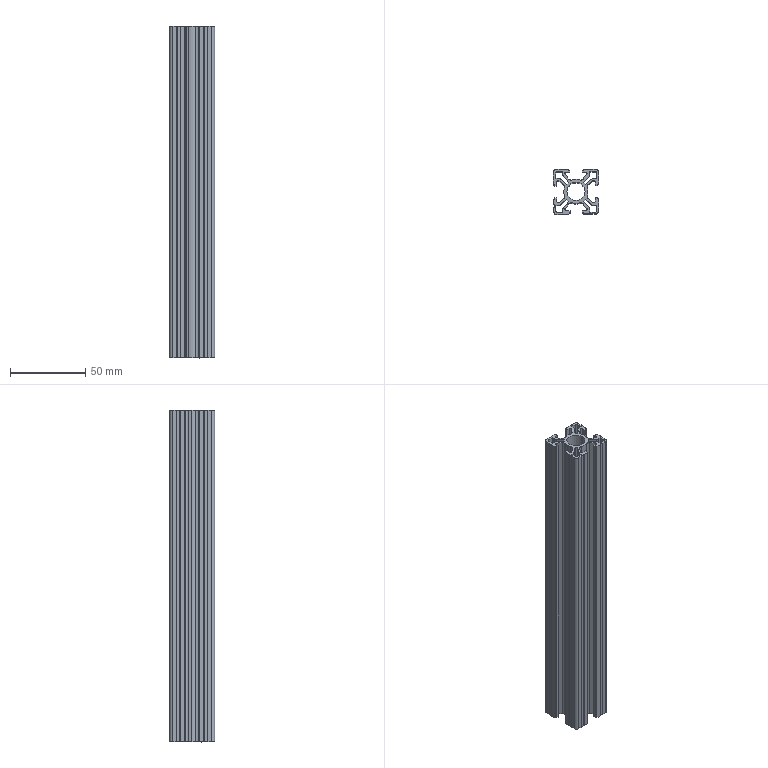Part | STEP file | 3030-200 | 1 solid | 154 faces | box 29.915 x 30.09 x 220 mm | volume 68984 mm3 | plane 110 | cylinder 44 | commonest cylinder face diameters 2 x15 4 x14 5 x8 16 x5 12 x2